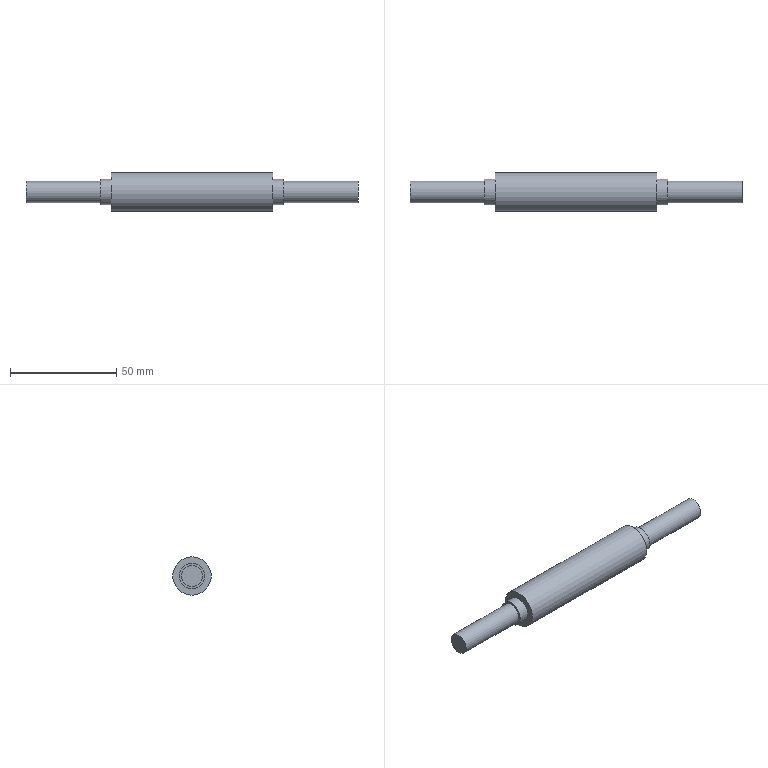Part | NX | 1 solid | 11 faces | box 156 x 18 x 18 mm | volume 25968 mm3 | plane 6 | cylinder 5 | commonest cylinder face diameters 10 x2 12 x2 18 x1
STEP:
#1=CARTESIAN_POINT('',(43.,0.,-6.));
#2=VERTEX_POINT('',#1);
#3=CARTESIAN_POINT('',(43.,0.,0.));
#4=DIRECTION('',(1.,0.,0.));
#5=DIRECTION('',(0.,0.,-1.));
#6=AXIS2_PLACEMENT_3D('',#3,#4,#5);
#7=CIRCLE('',#6,6.);
#8=EDGE_CURVE('',#2,#2,#7,.T.);
#9=ORIENTED_EDGE('',*,*,#8,.T.);
#10=EDGE_LOOP('',(#9));
#11=FACE_BOUND('',#10,.T.);
#12=CARTESIAN_POINT('',(43.,0.,-5.));
#13=VERTEX_POINT('',#12);
#14=CARTESIAN_POINT('',(43.,0.,0.));
#15=DIRECTION('',(1.,0.,0.));
#16=DIRECTION('',(0.,0.,-1.));
#17=AXIS2_PLACEMENT_3D('',#14,#15,#16);
#18=CIRCLE('',#17,5.);
#19=EDGE_CURVE('',#13,#13,#18,.T.);
#20=ORIENTED_EDGE('',*,*,#19,.F.);
#21=EDGE_LOOP('',(#20));
#22=FACE_BOUND('',#21,.T.);
#23=CARTESIAN_POINT('',(43.,0.,0.));
#24=DIRECTION('',(1.,0.,0.));
#25=DIRECTION('',(0.,0.,-1.));
#26=AXIS2_PLACEMENT_3D('',#23,#24,#25);
#27=PLANE('',#26);
#28=ADVANCED_FACE('',(#11,#22),#27,.T.);
#29=CARTESIAN_POINT('',(38.,0.,-9.));
#30=VERTEX_POINT('',#29);
#31=CARTESIAN_POINT('',(38.,0.,0.));
#32=DIRECTION('',(1.,0.,0.));
#33=DIRECTION('',(0.,0.,-1.));
#34=AXIS2_PLACEMENT_3D('',#31,#32,#33);
#35=CIRCLE('',#34,9.);
#36=EDGE_CURVE('',#30,#30,#35,.T.);
#37=ORIENTED_EDGE('',*,*,#36,.T.);
#38=EDGE_LOOP('',(#37));
#39=FACE_BOUND('',#38,.T.);
#40=CARTESIAN_POINT('',(38.,0.,-6.));
#41=VERTEX_POINT('',#40);
#42=CARTESIAN_POINT('',(38.,0.,0.));
#43=DIRECTION('',(1.,0.,0.));
#44=DIRECTION('',(0.,0.,-1.));
#45=AXIS2_PLACEMENT_3D('',#42,#43,#44);
#46=CIRCLE('',#45,6.);
#47=EDGE_CURVE('',#41,#41,#46,.T.);
#48=ORIENTED_EDGE('',*,*,#47,.F.);
#49=EDGE_LOOP('',(#48));
#50=FACE_BOUND('',#49,.T.);
#51=CARTESIAN_POINT('',(38.,0.,0.));
#52=DIRECTION('',(1.,0.,0.));
#53=DIRECTION('',(0.,0.,-1.));
#54=AXIS2_PLACEMENT_3D('',#51,#52,#53);
#55=PLANE('',#54);
#56=ADVANCED_FACE('',(#39,#50),#55,.T.);
#57=ORIENTED_EDGE('',*,*,#36,.F.);
#58=EDGE_LOOP('',(#57));
#59=FACE_BOUND('',#58,.T.);
#60=CARTESIAN_POINT('',(-38.,0.,-9.));
#61=VERTEX_POINT('',#60);
#62=CARTESIAN_POINT('',(-38.,0.,0.));
#63=DIRECTION('',(1.,0.,0.));
#64=DIRECTION('',(0.,0.,-1.));
#65=AXIS2_PLACEMENT_3D('',#62,#63,#64);
#66=CIRCLE('',#65,9.);
#67=EDGE_CURVE('',#61,#61,#66,.T.);
#68=ORIENTED_EDGE('',*,*,#67,.T.);
#69=EDGE_LOOP('',(#68));
#70=FACE_BOUND('',#69,.T.);
#71=CARTESIAN_POINT('',(38.,0.,0.));
#72=DIRECTION('',(-1.,0.,0.));
#73=DIRECTION('',(0.,0.,1.));
#74=AXIS2_PLACEMENT_3D('',#71,#72,#73);
#75=CYLINDRICAL_SURFACE('',#74,9.);
#76=ADVANCED_FACE('',(#59,#70),#75,.T.);
#77=CARTESIAN_POINT('',(-38.,0.,-6.));
#78=VERTEX_POINT('',#77);
#79=CARTESIAN_POINT('',(-38.,0.,0.));
#80=DIRECTION('',(1.,0.,0.));
#81=DIRECTION('',(0.,0.,-1.));
#82=AXIS2_PLACEMENT_3D('',#79,#80,#81);
#83=CIRCLE('',#82,6.);
#84=EDGE_CURVE('',#78,#78,#83,.T.);
#85=ORIENTED_EDGE('',*,*,#84,.T.);
#86=EDGE_LOOP('',(#85));
#87=FACE_BOUND('',#86,.T.);
#88=ORIENTED_EDGE('',*,*,#67,.F.);
#89=EDGE_LOOP('',(#88));
#90=FACE_BOUND('',#89,.T.);
#91=CARTESIAN_POINT('',(-38.,0.,0.));
#92=DIRECTION('',(1.,0.,0.));
#93=DIRECTION('',(0.,0.,-1.));
#94=AXIS2_PLACEMENT_3D('',#91,#92,#93);
#95=PLANE('',#94);
#96=ADVANCED_FACE('',(#87,#90),#95,.F.);
#97=ORIENTED_EDGE('',*,*,#8,.F.);
#98=EDGE_LOOP('',(#97));
#99=FACE_BOUND('',#98,.T.);
#100=ORIENTED_EDGE('',*,*,#47,.T.);
#101=EDGE_LOOP('',(#100));
#102=FACE_BOUND('',#101,.T.);
#103=CARTESIAN_POINT('',(43.,0.,0.));
#104=DIRECTION('',(-1.,0.,0.));
#105=DIRECTION('',(0.,0.,1.));
#106=AXIS2_PLACEMENT_3D('',#103,#104,#105);
#107=CYLINDRICAL_SURFACE('',#106,6.);
#108=ADVANCED_FACE('',(#99,#102),#107,.T.);
#109=CARTESIAN_POINT('',(78.,0.,-5.));
#110=VERTEX_POINT('',#109);
#111=CARTESIAN_POINT('',(78.,0.,0.));
#112=DIRECTION('',(1.,0.,0.));
#113=DIRECTION('',(0.,0.,-1.));
#114=AXIS2_PLACEMENT_3D('',#111,#112,#113);
#115=CIRCLE('',#114,5.);
#116=EDGE_CURVE('',#110,#110,#115,.T.);
#117=ORIENTED_EDGE('',*,*,#116,.F.);
#118=EDGE_LOOP('',(#117));
#119=FACE_BOUND('',#118,.T.);
#120=ORIENTED_EDGE('',*,*,#19,.T.);
#121=EDGE_LOOP('',(#120));
#122=FACE_BOUND('',#121,.T.);
#123=CARTESIAN_POINT('',(78.,0.,0.));
#124=DIRECTION('',(-1.,0.,0.));
#125=DIRECTION('',(0.,0.,1.));
#126=AXIS2_PLACEMENT_3D('',#123,#124,#125);
#127=CYLINDRICAL_SURFACE('',#126,5.);
#128=ADVANCED_FACE('',(#119,#122),#127,.T.);
#129=ORIENTED_EDGE('',*,*,#116,.T.);
#130=EDGE_LOOP('',(#129));
#131=FACE_BOUND('',#130,.T.);
#132=CARTESIAN_POINT('',(78.,0.,0.));
#133=DIRECTION('',(1.,0.,0.));
#134=DIRECTION('',(0.,0.,-1.));
#135=AXIS2_PLACEMENT_3D('',#132,#133,#134);
#136=PLANE('',#135);
#137=ADVANCED_FACE('',(#131),#136,.T.);
#138=CARTESIAN_POINT('',(-43.,0.,-6.));
#139=VERTEX_POINT('',#138);
#140=CARTESIAN_POINT('',(-43.,0.,0.));
#141=DIRECTION('',(1.,0.,0.));
#142=DIRECTION('',(0.,0.,-1.));
#143=AXIS2_PLACEMENT_3D('',#140,#141,#142);
#144=CIRCLE('',#143,6.);
#145=EDGE_CURVE('',#139,#139,#144,.T.);
#146=ORIENTED_EDGE('',*,*,#145,.T.);
#147=EDGE_LOOP('',(#146));
#148=FACE_BOUND('',#147,.T.);
#149=ORIENTED_EDGE('',*,*,#84,.F.);
#150=EDGE_LOOP('',(#149));
#151=FACE_BOUND('',#150,.T.);
#152=CARTESIAN_POINT('',(-43.,0.,0.));
#153=DIRECTION('',(1.,0.,0.));
#154=DIRECTION('',(0.,0.,-1.));
#155=AXIS2_PLACEMENT_3D('',#152,#153,#154);
#156=CYLINDRICAL_SURFACE('',#155,6.);
#157=ADVANCED_FACE('',(#148,#151),#156,.T.);
#158=CARTESIAN_POINT('',(-43.,0.,5.));
#159=VERTEX_POINT('',#158);
#160=CARTESIAN_POINT('',(-43.,0.,0.));
#161=DIRECTION('',(-1.,0.,0.));
#162=DIRECTION('',(0.,0.,1.));
#163=AXIS2_PLACEMENT_3D('',#160,#161,#162);
#164=CIRCLE('',#163,5.);
#165=EDGE_CURVE('',#159,#159,#164,.T.);
#166=ORIENTED_EDGE('',*,*,#165,.F.);
#167=EDGE_LOOP('',(#166));
#168=FACE_BOUND('',#167,.T.);
#169=ORIENTED_EDGE('',*,*,#145,.F.);
#170=EDGE_LOOP('',(#169));
#171=FACE_BOUND('',#170,.T.);
#172=CARTESIAN_POINT('',(-43.,0.,0.));
#173=DIRECTION('',(-1.,0.,0.));
#174=DIRECTION('',(0.,0.,-1.));
#175=AXIS2_PLACEMENT_3D('',#172,#173,#174);
#176=PLANE('',#175);
#177=ADVANCED_FACE('',(#168,#171),#176,.T.);
#178=CARTESIAN_POINT('',(-78.,0.,-5.));
#179=VERTEX_POINT('',#178);
#180=CARTESIAN_POINT('',(-78.,0.,0.));
#181=DIRECTION('',(1.,0.,0.));
#182=DIRECTION('',(0.,0.,-1.));
#183=AXIS2_PLACEMENT_3D('',#180,#181,#182);
#184=CIRCLE('',#183,5.);
#185=EDGE_CURVE('',#179,#179,#184,.T.);
#186=ORIENTED_EDGE('',*,*,#185,.T.);
#187=EDGE_LOOP('',(#186));
#188=FACE_BOUND('',#187,.T.);
#189=ORIENTED_EDGE('',*,*,#165,.T.);
#190=EDGE_LOOP('',(#189));
#191=FACE_BOUND('',#190,.T.);
#192=CARTESIAN_POINT('',(-78.,0.,0.));
#193=DIRECTION('',(1.,0.,0.));
#194=DIRECTION('',(0.,0.,-1.));
#195=AXIS2_PLACEMENT_3D('',#192,#193,#194);
#196=CYLINDRICAL_SURFACE('',#195,5.);
#197=ADVANCED_FACE('',(#188,#191),#196,.T.);
#198=ORIENTED_EDGE('',*,*,#185,.F.);
#199=EDGE_LOOP('',(#198));
#200=FACE_BOUND('',#199,.T.);
#201=CARTESIAN_POINT('',(-78.,0.,0.));
#202=DIRECTION('',(-1.,0.,0.));
#203=DIRECTION('',(0.,0.,-1.));
#204=AXIS2_PLACEMENT_3D('',#201,#202,#203);
#205=PLANE('',#204);
#206=ADVANCED_FACE('',(#200),#205,.T.);
#207=CLOSED_SHELL('',(#28,#56,#76,#96,#108,#128,#137,#157,#177,#197,#206));
#208=MANIFOLD_SOLID_BREP('',#207);
#209=(LENGTH_UNIT()NAMED_UNIT(*)SI_UNIT(.MILLI.,.METRE.));
#210=UNCERTAINTY_MEASURE_WITH_UNIT(LENGTH_MEASURE(0.00001),#209,'','');
#211=(NAMED_UNIT(*)PLANE_ANGLE_UNIT()SI_UNIT($,.RADIAN.));
#212=(NAMED_UNIT(*)SI_UNIT($,.STERADIAN.)SOLID_ANGLE_UNIT());
#213=(GEOMETRIC_REPRESENTATION_CONTEXT(3)GLOBAL_UNCERTAINTY_ASSIGNED_CONTEXT((#210))GLOBAL_UNIT_ASSIGNED_CONTEXT((#209,#211,#212))REPRESENTATION_CONTEXT('',''));
#214=ADVANCED_BREP_SHAPE_REPRESENTATION('',(#208),#213);